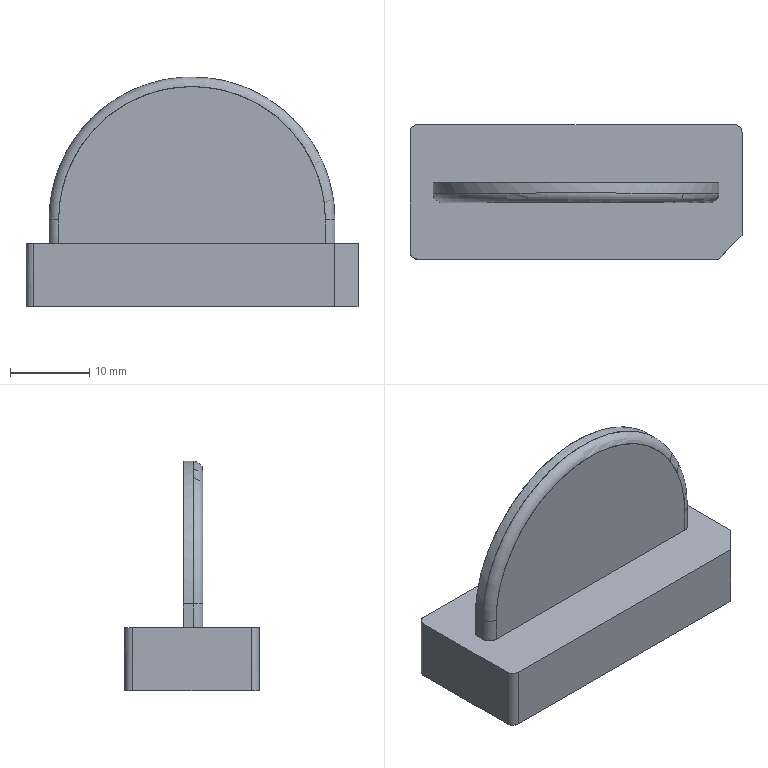NC program | PowerMill | posted with a generic post | part box 42 x 17 x 29.081 mm
Lines 13653 to 14348 of 145628:
N13750 M6
N13751 S8500 M03
N13752 G00 G90 X0.0 Y0.0
N13753 G43 Z9.702 H3
N13754
N13755 G05 P10000 R8
N13756 X30.8062 Y12.1216
N13757 Z-20.08
N13758 G01 Z-21.28 F360.0
N13759 X25.9374 Y10.0916 F600.0
N13760 X18.1163 Y6.5163
N13761 X18.4403 Y6.505
N13762 X18.724 Y6.4784
N13763 X19.0077 Y6.4366
N13764 X19.2914 Y6.3792
N13765 X19.575 Y6.3055
N13766 X19.8587 Y6.2148
N13767 X20.1424 Y6.1065
N13768 X20.4846 Y5.9502
N13769 X20.7098 Y5.8309
N13770 X20.9935 Y5.6604
N13771 X21.2772 Y5.4646
N13772 X21.3842 Y5.3835
N13773 X21.6144 Y5.1942
N13774 X21.8446 Y4.9815
N13775 X22.0059 Y4.8168
N13776 X22.221 Y4.5728
N13777 X22.412 Y4.3287
N13778 X22.4688 Y4.2501
N13779 X22.6566 Y3.9668
N13780 X22.8204 Y3.6834
N13781 X22.9794 Y3.3619
N13782 X23.0836 Y3.1168
N13783 X23.1867 Y2.8334
N13784 X23.2722 Y2.5501
N13785 X23.341 Y2.2667
N13786 X23.3941 Y1.9834
N13787 X23.4316 Y1.7001
N13788 X23.454 Y1.4167
N13789 X23.4612 Y0.85
N13790 X23.4598 Y-0.2833
N13791 X23.4491 Y-0.5667
N13792 X23.4257 Y-0.85
N13793 X23.3901 Y-1.1334
N13794 X23.3418 Y-1.4167
N13795 X23.2806 Y-1.7001
N13796 X23.2063 Y-1.9834
N13797 X23.1181 Y-2.2667
N13798 X22.9794 Y-2.6411
N13799 X22.8778 Y-2.8789
N13800 X22.7644 Y-3.1168
N13801 X22.6138 Y-3.4001
N13802 X22.412 Y-3.7346
N13803 X22.2375 Y-3.9924
N13804 X22.0438 Y-4.2501
N13805 X21.8446 Y-4.4906
N13806 X21.6981 Y-4.6537
N13807 X21.541 Y-4.8168
N13808 X21.2772 Y-5.0675
N13809 X21.0874 Y-5.2315
N13810 X20.8977 Y-5.3835
N13811 X20.7098 Y-5.5232
N13812 X20.4261 Y-5.715
N13813 X20.1424 Y-5.8871
N13814 X19.8019 Y-6.0686
N13815 X19.575 Y-6.1757
N13816 X19.2914 Y-6.2954
N13817 X19.0077 Y-6.3998
N13818 X18.6284 Y-6.5169
N13819 X18.4403 Y-6.5658
N13820 X18.1566 Y-6.6286
N13821 X17.8729 Y-6.6785
N13822 X17.5892 Y-6.7156
N13823 X17.3055 Y-6.7404
N13824 X16.7381 Y-6.7546
N13825 X-16.7381
N13826 X-17.3055 Y-6.7404
N13827 X-17.5892 Y-6.7156
N13828 X-17.8729 Y-6.6785
N13829 X-18.1566 Y-6.6286
N13830 X-18.4403 Y-6.5658
N13831 X-18.6284 Y-6.5169
N13832 X-19.0077 Y-6.3998
N13833 X-19.2914 Y-6.2954
N13834 X-19.575 Y-6.1757
N13835 X-19.8019 Y-6.0686
N13836 X-20.1424 Y-5.8871
N13837 X-20.4261 Y-5.715
N13838 X-20.7098 Y-5.5232
N13839 X-20.8977 Y-5.3835
N13840 X-21.0874 Y-5.2315
N13841 X-21.2772 Y-5.0675
N13842 X-21.541 Y-4.8168
N13843 X-21.6956 Y-4.6563
N13844 X-21.8446 Y-4.4906
N13845 X-22.0438 Y-4.2501
N13846 X-22.2375 Y-3.9924
N13847 X-22.4441 Y-3.6834
N13848 X-22.6139 Y-3.4001
N13849 X-22.7644 Y-3.1168
N13850 X-22.8777 Y-2.8789
N13851 X-23.0154 Y-2.5501
N13852 X-23.1181 Y-2.2667
N13853 X-23.2063 Y-1.9834
N13854 X-23.2807 Y-1.7001
N13855 X-23.3418 Y-1.4167
N13856 X-23.3902 Y-1.1334
N13857 X-23.4257 Y-0.85
N13858 X-23.4491 Y-0.5667
N13859 X-23.4598 Y-0.2833
N13860 X-23.4612 Y0.85
N13861 X-23.454 Y1.4167
N13862 X-23.4315 Y1.7001
N13863 X-23.3941 Y1.9834
N13864 X-23.3411 Y2.2667
N13865 X-23.2722 Y2.5501
N13866 X-23.1867 Y2.8334
N13867 X-23.0836 Y3.1168
N13868 X-22.9794 Y3.3619
N13869 X-22.8204 Y3.6834
N13870 X-22.6568 Y3.9668
N13871 X-22.4688 Y4.2501
N13872 X-22.412 Y4.3287
N13873 X-22.221 Y4.5728
N13874 X-22.0059 Y4.8168
N13875 X-21.8446 Y4.9815
N13876 X-21.6144 Y5.1942
N13877 X-21.3842 Y5.3835
N13878 X-21.2772 Y5.4646
N13879 X-20.9935 Y5.6604
N13880 X-20.7098 Y5.8309
N13881 X-20.4846 Y5.9502
N13882 X-20.1424 Y6.1065
N13883 X-19.8587 Y6.2148
N13884 X-19.575 Y6.3055
N13885 X-19.2914 Y6.3792
N13886 X-19.0077 Y6.4366
N13887 X-18.724 Y6.4784
N13888 X-18.4403 Y6.505
N13889 X-18.0992 Y6.5169
N13890 X18.1163 Y6.5163
N13891 G00 Z9.702
N13892 G05 P0
N13893 (---------------)
N13894 ( END TOOLPATH : 精公基准台01-基准面偏置-D10 )
N13895 (---------------)
N13896 ( START TOOLPATH : 精公基准台01-基准台侧光-D10 )
N13897 (---------------)
N13898 G00 X0.0 Y0.0 Z9.702
N13899 G05 P10000 R8
N13900 X25.9781 Y-14.7772
N13901 Z-27.98
N13902 G01 Z-29.18 F360.0
N13903 G03 X22.4426 Y-11.2416 I-1.7678 J1.7678 F600.0
N13904 G01 X21.6141 Y-12.0701
N13905 X21.6134 Y-12.0708
N13906 X21.6127 Y-12.0715
N13907 X21.395 Y-12.2789
N13908 X21.3937 Y-12.2801
N13909 X21.3923 Y-12.2814
N13910 X21.267 Y-12.3901
N13911 X21.2658 Y-12.3912
N13912 X21.2645 Y-12.3922
N13913 X21.0736 Y-12.5447
N13914 X21.0719 Y-12.5459
N13915 X21.0703 Y-12.5472
N13916 X20.8416 Y-12.7109
N13917 X20.8403 Y-12.7118
N13918 X20.8391 Y-12.7126
N13919 X20.7516 Y-12.7703
N13920 X20.75 Y-12.7713
N13921 X20.7484 Y-12.7723
N13922 X20.4322 Y-12.9599
N13923 X20.4304 Y-12.9609
N13924 X20.4286 Y-12.9619
N13925 X20.2935 Y-13.0328
N13926 X20.2922 Y-13.0335
N13927 X20.291 Y-13.0341
N13928 X20.1099 Y-13.1211
N13929 X20.1079 Y-13.122
N13930 X20.1059 Y-13.1229
N13931 X19.7898 Y-13.2542
N13932 X19.7874 Y-13.2552
N13933 X19.785 Y-13.2561
N13934 X19.4988 Y-13.3538
N13935 X19.4963 Y-13.3546
N13936 X19.4938 Y-13.3554
N13937 X19.1476 Y-13.4486
N13938 X19.145 Y-13.4493
N13939 X19.1423 Y-13.4499
N13940 X18.8262 Y-13.5123
N13941 X18.8237 Y-13.5128
N13942 X18.8211 Y-13.5132
N13943 X18.505 Y-13.5548
N13944 X18.5024 Y-13.5551
N13945 X18.4999 Y-13.5553
N13946 X18.1838 Y-13.5766
N13947 X18.1815 Y-13.5768
N13948 X18.1792
N13949 X17.863 Y-13.58
N13950 X17.8626
N13951 X17.8622
N13952 X-20.0753 Y-13.5794
N13953 X-20.0768
N13954 X-20.0783
N13955 X-20.3945 Y-13.5672
N13956 X-20.3966 Y-13.5671
N13957 X-20.3988 Y-13.5669
N13958 X-20.7149 Y-13.5377
N13959 X-20.717 Y-13.5375
N13960 X-20.7191 Y-13.5372
N13961 X-21.0352 Y-13.4912
N13962 X-21.0373 Y-13.4909
N13963 X-21.0395 Y-13.4905
N13964 X-21.3556 Y-13.4269
N13965 X-21.3576 Y-13.4264
N13966 X-21.3595 Y-13.426
N13967 X-21.636 Y-13.3557
N13968 X-21.6382 Y-13.3551
N13969 X-21.6403 Y-13.3545
N13970 X-21.9961 Y-13.2429
N13971 X-21.9983 Y-13.2421
N13972 X-22.0005 Y-13.2413
N13973 X-22.3167 Y-13.1213
N13974 X-22.3188 Y-13.1205
N13975 X-22.3209 Y-13.1196
N13976 X-22.6371 Y-12.9782
N13977 X-22.6392 Y-12.9772
N13978 X-22.6413 Y-12.9761
N13979 X-22.9574 Y-12.8121
N13980 X-22.959 Y-12.8112
N13981 X-22.9606 Y-12.8103
N13982 X-23.1254 Y-12.7151
N13983 X-23.1265 Y-12.7144
N13984 X-23.1276 Y-12.7138
N13985 X-23.2789 Y-12.6198
N13986 X-23.2805 Y-12.6188
N13987 X-23.282 Y-12.6178
N13988 X-23.5981 Y-12.401
N13989 X-23.6003 Y-12.3994
N13990 X-23.6024 Y-12.3978
N13991 X-23.9185 Y-12.1488
N13992 X-23.9198 Y-12.1477
N13993 X-23.9211 Y-12.1466
N13994 X-24.0054 Y-12.0742
N13995 X-24.0065 Y-12.0733
N13996 X-24.0075 Y-12.0723
N13997 X-24.2394 Y-11.858
N13998 X-24.2405 Y-11.857
N13999 X-24.2416 Y-11.8559
N14000 X-24.3438 Y-11.7541
N14001 X-24.3449 Y-11.753
N14002 X-24.3459 Y-11.7518
N14003 X-24.5599 Y-11.5215
N14004 X-24.561 Y-11.5203
N14005 X-24.562 Y-11.5192
N14006 X-24.6356 Y-11.4333
N14007 X-24.6366 Y-11.4322
N14008 X-24.6375 Y-11.4311
N14009 X-24.88 Y-11.1264
N14010 X-24.8817 Y-11.1242
N14011 X-24.8832 Y-11.122
N14012 X-25.1097 Y-10.7944
N14013 X-25.1107 Y-10.793
N14014 X-25.1117 Y-10.7914
N14015 X-25.2014 Y-10.6483
N14016 X-25.2021 Y-10.6472
N14017 X-25.2027 Y-10.6461
N14018 X-25.3034 Y-10.473
N14019 X-25.3043 Y-10.4714
N14020 X-25.3052 Y-10.4698
N14021 X-25.4703 Y-10.1537
N14022 X-25.4713 Y-10.1516
N14023 X-25.4723 Y-10.1495
N14024 X-25.6144 Y-9.8333
N14025 X-25.6153 Y-9.8312
N14026 X-25.6162 Y-9.8291
N14027 X-25.737 Y-9.5129
N14028 X-25.7378 Y-9.5108
N14029 X-25.7385 Y-9.5087
N14030 X-25.8396 Y-9.1926
N14031 X-25.8403 Y-9.1905
N14032 X-25.8408 Y-9.1884
N14033 X-25.9231 Y-8.8722
N14034 X-25.9236 Y-8.87
N14035 X-25.9241 Y-8.8678
N14036 X-25.9876 Y-8.5517
N14037 X-25.988 Y-8.5497
N14038 X-25.9883 Y-8.5478
N14039 X-26.0357 Y-8.2317
N14040 X-26.036 Y-8.2294
N14041 X-26.0363 Y-8.2271
N14042 X-26.0653 Y-7.911
N14043 X-26.0655 Y-7.909
N14044 X-26.0656 Y-7.9071
N14045 X-26.0792 Y-7.5909
N14046 Y-7.5892
N14047 Y-7.5875
N14048 Y7.5875
N14049 Y7.5891
N14050 Y7.5907
N14051 X-26.0664 Y7.9069
N14052 X-26.0662 Y7.909
N14053 X-26.0661 Y7.9112
N14054 X-26.0362 Y8.2273
N14055 X-26.036 Y8.2294
N14056 X-26.0357 Y8.2315
N14057 X-25.989 Y8.5476
N14058 X-25.9887 Y8.5498
N14059 X-25.9883 Y8.5519
N14060 X-25.924 Y8.868
N14061 X-25.9236 Y8.8701
N14062 X-25.9231 Y8.8722
N14063 X-25.8433 Y9.1794
N14064 X-25.8427 Y9.1815
N14065 X-25.8421 Y9.1836
N14066 X-25.7384 Y9.5087
N14067 X-25.7377 Y9.5108
N14068 X-25.7369 Y9.5129
N14069 X-25.6162 Y9.8291
N14070 X-25.6153 Y9.8312
N14071 X-25.6144 Y9.8334
N14072 X-25.4721 Y10.1495
N14073 X-25.4711 Y10.1516
N14074 X-25.4701 Y10.1537
N14075 X-25.3052 Y10.4698
N14076 X-25.3043 Y10.4714
N14077 X-25.3034 Y10.473
N14078 X-25.2027 Y10.6461
N14079 X-25.2021 Y10.6472
N14080 X-25.2014 Y10.6483
N14081 X-25.1119 Y10.7914
N14082 X-25.1109 Y10.7929
N14083 X-25.1099 Y10.7944
N14084 X-24.8918 Y11.1105
N14085 X-24.8903 Y11.1127
N14086 X-24.8887 Y11.1148
N14087 X-24.6383 Y11.4309
N14088 X-24.6372 Y11.4323
N14089 X-24.6361 Y11.4336
N14090 X-24.5618 Y11.5195
N14091 X-24.5609 Y11.5206
N14092 X-24.5599 Y11.5216
N14093 X-24.3459 Y11.7519
N14094 X-24.3449 Y11.753
N14095 X-24.3438 Y11.7541
N14096 X-24.2416 Y11.8559
N14097 X-24.2405 Y11.8569
N14098 X-24.2394 Y11.858
N14099 X-24.0073 Y12.0723
N14100 X-24.0062 Y12.0734
N14101 X-24.0049 Y12.0744
N14102 X-23.9209 Y12.146
N14103 X-23.9198 Y12.147
N14104 X-23.9186 Y12.1479
N14105 X-23.6097 Y12.3924
N14106 X-23.6075 Y12.3941
N14107 X-23.6053 Y12.3956
N14108 X-23.282 Y12.6178
N14109 X-23.2805 Y12.6188
N14110 X-23.2789 Y12.6198
N14111 X-23.1276 Y12.7138
N14112 X-23.1266 Y12.7144
N14113 X-23.1254 Y12.7151
N14114 X-22.9606 Y12.8103
N14115 X-22.959 Y12.8112
N14116 X-22.9574 Y12.8121
N14117 X-22.6413 Y12.9763
N14118 X-22.6392 Y12.9773
N14119 X-22.6371 Y12.9783
N14120 X-22.3209 Y13.1196
N14121 X-22.3188 Y13.1205
N14122 X-22.3167 Y13.1213
N14123 X-22.0005 Y13.2414
N14124 X-21.9984 Y13.2421
N14125 X-21.9963 Y13.2429
N14126 X-21.6802 Y13.3432
N14127 X-21.6781 Y13.3438
N14128 X-21.676 Y13.3444
N14129 X-21.3598 Y13.426
N14130 X-21.3576 Y13.4265
N14131 X-21.3554 Y13.427
N14132 X-21.0393 Y13.4897
N14133 X-21.0373 Y13.4901
N14134 X-21.0354 Y13.4904
N14135 X-20.7193 Y13.5372
N14136 X-20.717 Y13.5375
N14137 X-20.7147 Y13.5377
N14138 X-20.3985 Y13.566
N14139 X-20.3966 Y13.5662
N14140 X-20.3947 Y13.5663
N14141 X-20.0786 Y13.5794
N14142 X-20.0769
N14143 X-20.0753
N14144 X-0.3161
N14145 X20.0753
N14146 X20.0768
N14147 X20.0783
N14148 X20.3945 Y13.5672
N14149 X20.3966 Y13.5671
N14150 X20.3988 Y13.5669
N14151 X20.7149 Y13.5377
N14152 X20.717 Y13.5375
N14153 X20.7191 Y13.5372
N14154 X21.0352 Y13.4912
N14155 X21.0373 Y13.4909
N14156 X21.0395 Y13.4905
N14157 X21.3556 Y13.4269
N14158 X21.3576 Y13.4264
N14159 X21.3595 Y13.426
N14160 X21.636 Y13.3557
N14161 X21.6382 Y13.3551
N14162 X21.6403 Y13.3545
N14163 X21.9961 Y13.2428
N14164 X21.9983 Y13.2421
N14165 X22.0005 Y13.2413
N14166 X22.3167 Y13.1213
N14167 X22.3188 Y13.1205
N14168 X22.3209 Y13.1196
N14169 X22.6371 Y12.9782
N14170 X22.6392 Y12.9772
N14171 X22.6413 Y12.9761
N14172 X22.9574 Y12.8121
N14173 X22.959 Y12.8112
N14174 X22.9606 Y12.8103
N14175 X23.1254 Y12.7151
N14176 X23.1266 Y12.7144
N14177 X23.1276 Y12.7138
N14178 X23.2789 Y12.6198
N14179 X23.2805 Y12.6188
N14180 X23.282 Y12.6178
N14181 X23.5981 Y12.401
N14182 X23.6003 Y12.3994
N14183 X23.6024 Y12.3978
N14184 X23.9185 Y12.1488
N14185 X23.9198 Y12.1477
N14186 X23.9211 Y12.1466
N14187 X24.0054 Y12.0742
N14188 X24.0065 Y12.0733
N14189 X24.0075 Y12.0723
N14190 X24.2394 Y11.858
N14191 X24.2405 Y11.857
N14192 X24.2416 Y11.8559
N14193 X24.3438 Y11.7541
N14194 X24.3449 Y11.753
N14195 X24.3459 Y11.7518
N14196 X24.5599 Y11.5215
N14197 X24.561 Y11.5203
N14198 X24.562 Y11.5192
N14199 X24.6356 Y11.4333
N14200 X24.6366 Y11.4322
N14201 X24.6375 Y11.4311
N14202 X24.88 Y11.1264
N14203 X24.8817 Y11.1242
N14204 X24.8832 Y11.122
N14205 X25.1097 Y10.7944
N14206 X25.1107 Y10.793
N14207 X25.1117 Y10.7914
N14208 X25.2014 Y10.6483
N14209 X25.2021 Y10.6472
N14210 X25.2027 Y10.6461
N14211 X25.3034 Y10.473
N14212 X25.3043 Y10.4714
N14213 X25.3052 Y10.4698
N14214 X25.4703 Y10.1537
N14215 X25.4713 Y10.1516
N14216 X25.4723 Y10.1495
N14217 X25.6144 Y9.8333
N14218 X25.6153 Y9.8312
N14219 X25.6162 Y9.8291
N14220 X25.737 Y9.5129
N14221 X25.7378 Y9.5108
N14222 X25.7385 Y9.5087
N14223 X25.8396 Y9.1926
N14224 X25.8403 Y9.1905
N14225 X25.8408 Y9.1884
N14226 X25.9231 Y8.8722
N14227 X25.9236 Y8.87
N14228 X25.9241 Y8.8678
N14229 X25.9876 Y8.5517
N14230 X25.988 Y8.5497
N14231 X25.9883 Y8.5478
N14232 X26.0357 Y8.2317
N14233 X26.036 Y8.2294
N14234 X26.0363 Y8.2271
N14235 X26.0653 Y7.911
N14236 X26.0655 Y7.909
N14237 X26.0656 Y7.9071
N14238 X26.0792 Y7.5909
N14239 Y7.5892
N14240 Y7.5875
N14241 X26.08 Y-5.3745
N14242 Y-5.3749
N14243 Y-5.3754
N14244 X26.0764 Y-5.6915
N14245 X26.0763 Y-5.6939
N14246 X26.0762 Y-5.6962
N14247 X26.0541 Y-6.0123
N14248 X26.0539 Y-6.0149
N14249 X26.0536 Y-6.0174
N14250 X26.0111 Y-6.3336
N14251 X26.0107 Y-6.3361
N14252 X26.0103 Y-6.3386
N14253 X25.947 Y-6.6548
N14254 X25.9464 Y-6.6573
N14255 X25.9458 Y-6.6598
N14256 X25.8608 Y-6.976
N14257 X25.8601 Y-6.9785
N14258 X25.8593 Y-6.981
N14259 X25.7514 Y-7.2972
N14260 X25.7505 Y-7.2997
N14261 X25.7495 Y-7.3022
N14262 X25.6172 Y-7.6184
N14263 X25.6163 Y-7.6204
N14264 X25.6154 Y-7.6224
N14265 X25.5217 Y-7.8153
N14266 X25.5211 Y-7.8166
N14267 X25.5204 Y-7.8178
N14268 X25.455 Y-7.9411
N14269 X25.4541 Y-7.9429
N14270 X25.453 Y-7.9447
N14271 X25.2643 Y-8.2608
N14272 X25.2633 Y-8.2624
N14273 X25.2622 Y-8.2641
N14274 X25.2002 Y-8.3574
N14275 X25.1994 Y-8.3587
N14276 X25.1985 Y-8.3599
N14277 X25.0377 Y-8.5827
N14278 X25.0364 Y-8.5844
N14279 X25.0351 Y-8.5861
N14280 X24.8798 Y-8.7793
N14281 X24.8787 Y-8.7805
N14282 X24.8777 Y-8.7818
N14283 X24.7702 Y-8.9047
N14284 X24.769 Y-8.9061
N14285 X24.7677 Y-8.9074
N14286 X24.559 Y-9.1251
N14287 X24.5585 Y-9.1258
N14288 X24.5579 Y-9.1264
N14289 X22.4426 Y-11.2416
N14290 G03 X25.9781 Y-14.7772 I1.7677 J-1.7678
N14291 G01 X25.9267 Y-14.7155
N14292 G03 X22.3911 Y-11.18 I-1.7678 J1.7678
N14293 G01 X21.5576 Y-12.0135
N14294 X21.3398 Y-12.221
N14295 X21.2146 Y-12.3297
N14296 X21.0237 Y-12.4821
N14297 X20.795 Y-12.6458
N14298 X20.7075 Y-12.7035
N14299 X20.3914 Y-12.8911
N14300 X20.2563 Y-12.962
N14301 X20.0753 Y-13.049
N14302 X19.7591 Y-13.1804
N14303 X19.473 Y-13.2781
N14304 X19.1268 Y-13.3714
N14305 X18.8107 Y-13.4339
N14306 X18.4945 Y-13.4755
N14307 X18.1784 Y-13.4968
N14308 X17.8622 Y-13.5
N14309 X-19.443
N14310 X-20.0753 Y-13.4994
N14311 X-20.3914 Y-13.4872
N14312 X-20.7075 Y-13.458
N14313 X-21.0237 Y-13.412
N14314 X-21.3398 Y-13.3484
N14315 X-21.6163 Y-13.2781
N14316 X-21.9721 Y-13.1665
N14317 X-22.2883 Y-13.0465
N14318 X-22.6044 Y-12.9051
N14319 X-22.9206 Y-12.7411
N14320 X-23.0854 Y-12.6458
N14321 X-23.2367 Y-12.5518
N14322 X-23.5529 Y-12.335
N14323 X-23.869 Y-12.0859
N14324 X-23.9532 Y-12.0135
N14325 X-24.1851 Y-11.7992
N14326 X-24.2873 Y-11.6974
N14327 X-24.5013 Y-11.4671
N14328 X-24.5749 Y-11.3812
N14329 X-24.8174 Y-11.0765
N14330 X-25.0439 Y-10.749
N14331 X-25.1336 Y-10.6058
N14332 X-25.2343 Y-10.4328
N14333 X-25.3993 Y-10.1167
N14334 X-25.5415 Y-9.8005
N14335 X-25.6623 Y-9.4844
N14336 X-25.7634 Y-9.1682
N14337 X-25.8457 Y-8.8521
N14338 X-25.9092 Y-8.5359
N14339 X-25.9566 Y-8.2198
N14340 X-25.9856 Y-7.9036
N14341 X-25.9992 Y-7.5875
N14342 X-26.0 Y-7.2714
N14343 Y7.2714
N14344 X-25.9992 Y7.5875
N14345 X-25.9864 Y7.9036
N14346 X-25.9566 Y8.2198
N14347 X-25.9099 Y8.5359
N14348 X-25.8456 Y8.8521
N14349 X-25.7659 Y9.1593
N14350 X-25.6622 Y9.4844
N14351 X-25.5415 Y9.8005
N14352 X-25.3992 Y10.1167
N14353 X-25.2343 Y10.4328
N14354 X-25.1336 Y10.6058
N14355 X-25.044 Y10.749
N14356 X-24.8259 Y11.0651
N14357 X-24.5756 Y11.3812
N14358 X-24.5013 Y11.4672
N14359 X-24.2873 Y11.6974
N14360 X-24.1851 Y11.7992
N14361 X-23.9531 Y12.0135
N14362 X-23.869 Y12.0851
N14363 X-23.56 Y12.3297
N14364 X-23.2367 Y12.5518
N14365 X-23.0854 Y12.6458
N14366 X-22.9206 Y12.7411
N14367 X-22.6044 Y12.9053
N14368 X-22.2883 Y13.0465
N14369 X-21.9721 Y13.1666
N14370 X-21.656 Y13.2669
N14371 X-21.3398 Y13.3485
N14372 X-21.0237 Y13.4113
N14373 X-20.7075 Y13.4581
N14374 X-20.3914 Y13.4864
N14375 X-20.0753 Y13.4994
N14376 X-19.7591 Y13.5
N14377 X-0.3161
N14378 X19.1268
N14379 X20.0753 Y13.4994
N14380 X20.3914 Y13.4872
N14381 X20.7075 Y13.458
N14382 X21.0237 Y13.412
N14383 X21.3398 Y13.3484
N14384 X21.6163 Y13.2781
N14385 X21.9721 Y13.1665
N14386 X22.2883 Y13.0465
N14387 X22.6044 Y12.9051
N14388 X22.9206 Y12.7411
N14389 X23.0854 Y12.6458
N14390 X23.2367 Y12.5518
N14391 X23.5529 Y12.335
N14392 X23.869 Y12.0859
N14393 X23.9532 Y12.0135
N14394 X24.1851 Y11.7992
N14395 X24.2873 Y11.6974
N14396 X24.5013 Y11.4671
N14397 X24.5749 Y11.3812
N14398 X24.8174 Y11.0765
N14399 X25.0439 Y10.749
N14400 X25.1336 Y10.6058
N14401 X25.2343 Y10.4328
N14402 X25.3993 Y10.1167
N14403 X25.5415 Y9.8005
N14404 X25.6623 Y9.4844
N14405 X25.7634 Y9.1682
N14406 X25.8457 Y8.8521
N14407 X25.9092 Y8.5359
N14408 X25.9566 Y8.2198
N14409 X25.9856 Y7.9036
N14410 X25.9992 Y7.5875
N14411 X26.0 Y7.2714
N14412 Y-5.3745
N14413 X25.9964 Y-5.6906
N14414 X25.9743 Y-6.0068
N14415 X25.9318 Y-6.3229
N14416 X25.8685 Y-6.6391
N14417 X25.7836 Y-6.9552
N14418 X25.6757 Y-7.2714
N14419 X25.5434 Y-7.5875
N14420 X25.4497 Y-7.7804
N14421 X25.3844 Y-7.9036
N14422 X25.1956 Y-8.2198
N14423 X25.1336 Y-8.3131
N14424 X24.9728 Y-8.5359
N14425 X24.8174 Y-8.7291
N14426 X24.7099 Y-8.8521
N14427 X24.5013 Y-9.0698
N14428 X22.3911 Y-11.18
N14429 G03 X25.9267 Y-14.7155 I1.7678 J-1.7677
N14430 G00 Z9.702
N14431 G05 P0
N14432 (---------------)
N14433 ( END TOOLPATH : 精公基准台01-基准台侧光-D10 )
N14434 (---------------)
N14435
N14436 M05
N14437 G53 Z0.0
N14438 (---------------)
N14439 ( START TOOLPATH : 精公精光01-平行-R2 )
N14440 (---------------)
N14441 ( TOOL NO.    :7 )
N14442 ( TOOL TYPE   : BALLNOSED)
N14443 ( TOOL ID     : R2_1_1)
N14444 ( TOOL DIA    : 4.0 LENGTH 75.4)
N14445 T7